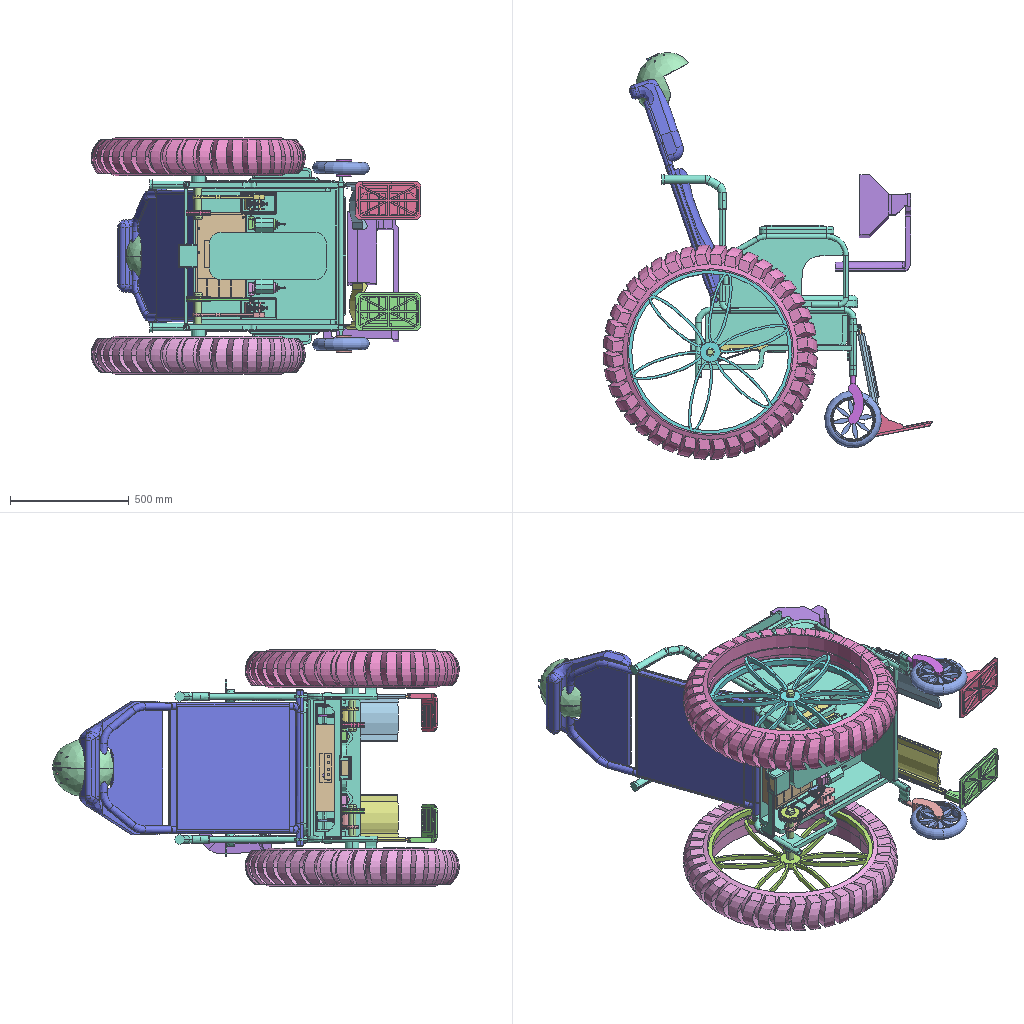Assembly | SolidWorks | 32 different items | 147 placed | box 1385 x 1709 x 995 mm
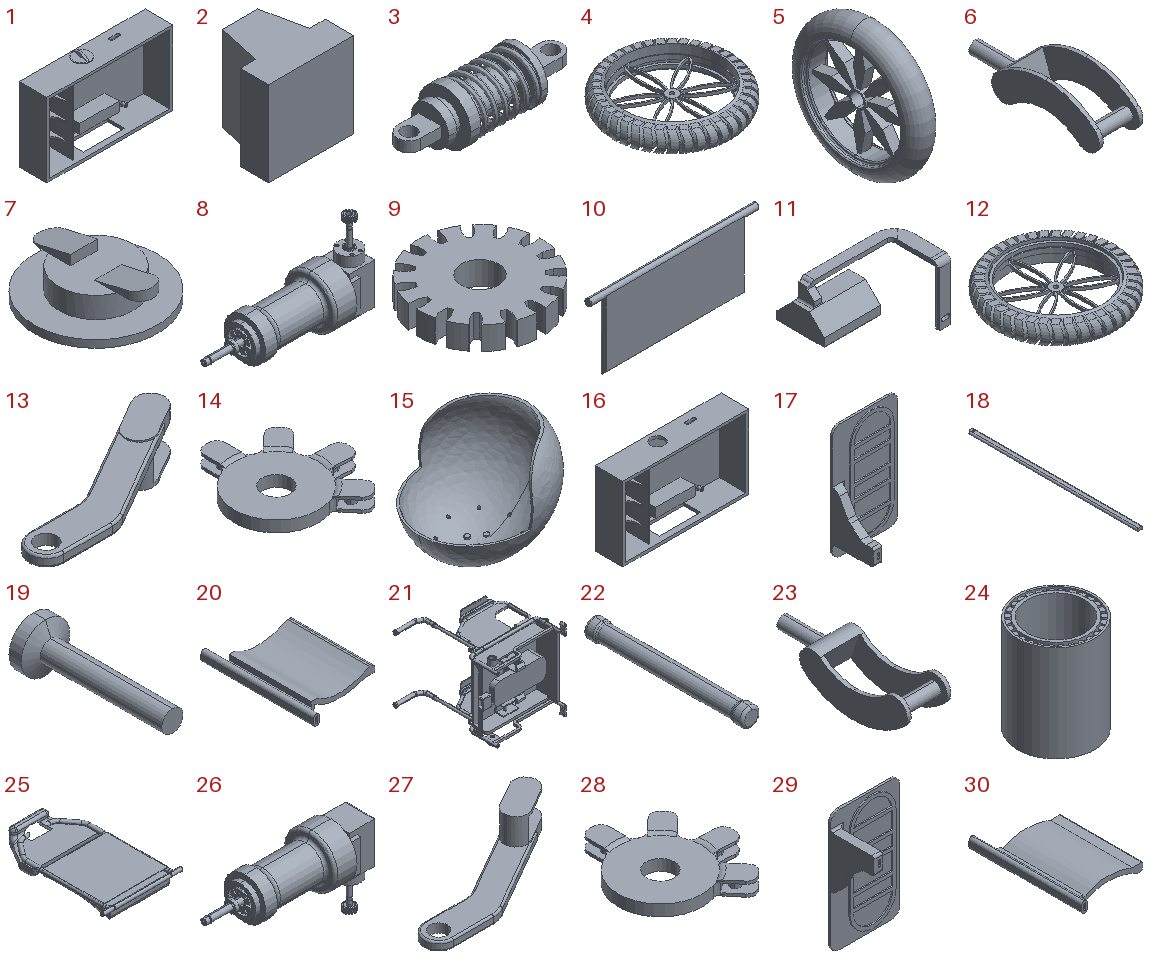Parts list (item | name | quantity | parent item | size | volume | features):
1 | (subassembly) | x1 | - | 366 x 80 x 226.454 mm | 995673 mm3 | features Fillet 2
2 | - | x109 | - | 6 x 5 x 6 mm | 128.419 mm3 | features Extrusion 1
3 | - | x2 | - | 79 x 25 x 25 mm | 12692 mm3 | features Extrusion 1, Helix 1, Revolution 1, Sweep 1
4 | - | x1 | - | 900 x 900 x 159.998 mm | 29745810 mm3 | features ICE 5, CirPattern 4, BossThin 1, ExtruThin 1, Fillet 1, RefAxis 1, RevCut 1, Revolution 1
5 | - | x2 | - | 50 x 239.862 x 239.862 mm | 1028496 mm3 | features ICE 3, CirPattern 1, Fillet 1, Revolution 1
6 | - | x1 | - | 69 x 230 x 64.48 mm | 170507 mm3 | features ICE 4, Extrusion 1
7 | - | x1 | in 1 | 50 x 50 x 22.954 mm | 14058 mm3 | features ICE 5, Extrusion 1
8 | - | x1 | - | 159.542 x 53.214 x 87.607 mm | 170177 mm3 | features ICE 20, Fillet 3, HoleWzd 2, CirPattern 1, Revolution 1
9 | - | x1 | - | 26.541 x 26.503 x 5 mm | 2075 mm3 | features ICE 4, CirPattern 1, Extrusion 1
10 | - | x1 | - | 79.5 x 3 x 34.5 mm | 6609 mm3 | features Fillet 2, Chamfer 1, Extrusion 1, ICE 1
11 | - | x1 | - | 546.764 x 377.712 x 317.016 mm | 9050376 mm3 | features ICE 10, Fillet 8, Chamfer 2, Sweep 2, Extrusion 1
12 | - | x1 | - | 900 x 900 x 159.998 mm | 29746479 mm3 | features MirrorStock 1
13 | - | x1 | - | 287.553 x 138.722 x 62 mm | 231304 mm3 | features ICE 4, Extrusion 1, Fillet 1, LPattern 1
14 | - | x1 | - | 80.013 x 90.67 x 10 mm | 26380 mm3 | features ICE 4, Fillet 2, CirPattern 1, Extrusion 1
15 | - | x1 | - | 256.913 x 240.018 x 217.091 mm | 479956 mm3 | features ICE 4, Bending 1, Fillet 1, Revolution 1, Shell 1
16 | - | x1 | in 1 | 366 x 80 x 216 mm | 981778 mm3 | features ICE 13, BossThin 1, Extrusion 1, LPattern 1
17 | - | x1 | - | 160 x 115 x 280 mm | 478660 mm3 | features Fillet 5, ICE 4, BossThin 2, Chamfer 1, Extrusion 1
18 | - | x2 | - | 14 x 400 x 6 mm | 30370 mm3 | features ICE 2, Extrusion 1
19 | - | x1 | - | 8 x 22.9 x 8 mm | 317.503 mm3 | features Revolution 1
20 | - | x1 | - | 194.613 x 302 x 37.008 mm | 615517 mm3 | features ExtruThin 1, ICE 1
21 | - | x1 | - | 838.639 x 850 x 766 mm | 46006837 mm3 | features ICE 30, Fillet 19, MirrorPattern 15, Cut 6, Sweep 4, BossThin 2, Chamfer 2, LPattern 2, MirrorSolid 1
22 | - | x2 | - | 35 x 300 x 35 mm | 221656 mm3 | features Fillet 3, Extrusion 1, ICE 1, MirrorPattern 1
23 | - | x1 | - | 69 x 230 x 64.48 mm | 170507 mm3 | features MirrorStock 1
24 | - | x2 | - | 40 x 40 x 50 mm | 21973 mm3 | features ICE 2, Extrusion 1
25 | - | x1 | - | 660 x 980.123 x 156.408 mm | 26120441 mm3 | features ICE 6, Fillet 4, Sweep 2, BossThin 1, Cut 1
26 | - | x1 | - | 159.542 x 53.214 x 87.607 mm | 170177 mm3 | features MirrorStock 1
27 | - | x1 | - | 287.553 x 138.722 x 62 mm | 231304 mm3 | features MirrorStock 1
28 | - | x1 | - | 80.013 x 90.67 x 10 mm | 26380 mm3 | features MirrorStock 1
29 | - | x1 | - | 160 x 115 x 280 mm | 478660 mm3 | features MirrorStock 1
30 | - | x1 | - | 194.613 x 302 x 37.008 mm | 615517 mm3 | features MirrorStock 1
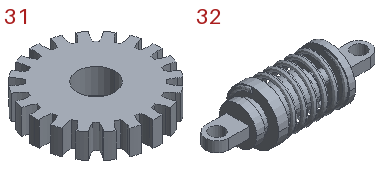31 | - | x2 | - | 99.281 x 99.281 x 20 mm | 114594 mm3 | features ICE 2, CirPattern 1, Cut 1, Extrusion 1
32 | - | x2 | - | 79 x 25 x 25 mm | 12692 mm3 | features MirrorStock 1
Mates (type | each side: item.copy, entity, surface, feature):
In the top assembly
Concentric | 6.1 face cylinder Boss-Extrude2 | 5.1 face cylinder Boss-Extrude2
Width | 6.1 face plane Boss-Extrude1 | 6.1 face plane Boss-Extrude1 | 5.1 face plane Boss-Extrude1 | 5.1 face plane Boss-Extrude1
Width | 21.1 face plane Boss-Extrude5 | 21.1 face plane Boss-Extrude5 | 18.1 face plane Boss-Extrude1 | 18.1 face plane Boss-Extrude1
Concentric | 21.1 face cylinder Cut-Extrude1 | 18.1 face cylinder Cut-Extrude2
DistanceDim | 6.1 face plane Boss-Extrude3 | 21.1 face plane Mirror3
Concentric | 18.1 face cylinder Cut-Extrude2 | 19.1 face cylinder Revolve1
DistanceDim | 19.1 face plane Revolve1 | 21.1 face plane Boss-Extrude5
Coincident | 17.1 face plane Cut-Extrude3 | 18.2 face plane Boss-Extrude1
Concentric | 17.1 face cylinder Cut-Extrude3 | 18.2 face cylinder Boss-Extrude1
DistanceDim | 17.1 face plane Cut-Extrude3 | 18.2 face plane Boss-Extrude1
Coincident | 18.1 face plane Boss-Extrude1 | 20.1 face plane Extrude-Thin1
Concentric | 18.1 face cylinder Boss-Extrude1 | 20.1 face cylinder Extrude-Thin1
DistanceDim | 29.1 face plane Footboard_Mirror | 20.1 face plane Extrude-Thin1
Concentric | 6.1 face cylinder Boss-Extrude3 | 21.1 face cylinder Mirror3
Concentric | 4.1 face cylinder Boss-Extrude1 | 21.1 face cylinder Mirror8
Concentric | 21.1 face cylinder Mirror8 | 24.1 face cylinder Boss-Extrude3
DistanceDim | 24.1 face plane Boss-Extrude1 | 21.1 face plane Boss-Extrude8
Concentric | 21.1 face cylinder Boss-Extrude15 | 25.1 face cylinder
Width | 25.1 face plane | 25.1 face plane | 21.1 face plane Mirror22 | 21.1 face plane Boss-Extrude15
DistanceDim | 4.1 face plane Boss-Extrude1 | 21.1 face plane Mirror7
Concentric | 4.1 face cylinder Boss-Extrude1 | 22.1 face cylinder Boss-Extrude1
Concentric | 21.1 face cylinder Cut-Extrude5 | 10.1 face cylinder Boss-Extrude2
Width | 21.1 face plane Boss-Extrude16 | 21.1 face plane Boss-Extrude16 | 10.1 face plane Boss-Extrude1 | 10.1 face plane Boss-Extrude1
Width | 11.1 face plane Cut-Extrude3 | 11.1 face plane Cut-Extrude3 | 21.1 face plane Sweep-Thin2 | 21.1 face plane Sweep-Thin2
DistanceDim | 4.1 face plane Boss-Extrude1 | 22.1 face plane Mirror1
Concentric | 22.1 face cylinder Boss-Extrude1 | 13.1 face cylinder Cut-Extrude1
DistanceDim | 21.1 face plane Boss-Extrude8 | 13.1 face plane Boss-Extrude1
Concentric | 3.1 face cylinder Boss-Extrude1 | 13.1 face cylinder Boss-Extrude3
Concentric | 13.1 face cylinder LPattern1 | 3.2 face cylinder Boss-Extrude1
Width | 13.1 face plane Cut-Extrude3 | 13.1 face plane Cut-Extrude3 | 3.2 face plane Boss-Extrude1 | 3.2 face plane Boss-Extrude1
Concentric | 22.1 face cylinder Boss-Extrude2 | 31.1 face cylinder Cut-Extrude1
Concentric | 3.1 face cylinder Boss-Extrude1 | 14.1 face cylinder CirPattern6
Concentric | 3.2 face cylinder Boss-Extrude1 | 14.1 face cylinder CirPattern6
Coincident | 21.1 face plane Cut-Extrude11 | 8.1 face plane Boss-Extrude3
Coincident | 21.1 face plane Boss-Extrude23 | 8.1 face plane Revolve1
Width | 14.1 face plane CirPattern6 | 14.1 face plane CirPattern6 | 3.2 face plane Boss-Extrude1 | 3.2 face plane Boss-Extrude1
Width | 13.1 face plane Cut-Extrude3 | 13.1 face plane Cut-Extrude3 | 3.1 face plane Boss-Extrude1 | 3.1 face plane Boss-Extrude1
Concentric | 21.1 face cylinder Mirror25 | 14.1 face cylinder Cut-Extrude1
DistanceDim | 13.1 face plane Boss-Extrude1 | 31.1 face plane Boss-Extrude1
DistanceDim | 16.1 face plane Boss-Extrude1 | 21.1 face plane Boss-Extrude18
Coincident | 21.1 face plane Boss-Extrude18 | 16.1 face plane Boss-Extrude1
Width | 16.1 face plane Boss-Extrude1 | 16.1 face plane Boss-Extrude1 | 21.1 face plane Boss-Extrude26 | 21.1 face plane Boss-Extrude26
Width | 31.1 face plane Boss-Extrude1 | 31.1 face plane Boss-Extrude1 | 9.1 face plane Boss-Extrude1 | 9.1 face plane Boss-Extrude1
Concentric | 9.1 face cylinder Cut-Extrude4 | assembly select_type:11
Concentric | 31.1 face cylinder Cut-Extrude1 | assembly select_type:11
BeltDim | 9.1 face cylinder Cut-Extrude3 | 31.1 face cylinder Cut-Extrude4
RackPinionDim | 2.1 edge | 9.1 face cylinder Cut-Extrude3
Coincident | 15.1 plane | assembly plane
Lock | 25.1 select_type:0 | 15.1 select_type:0
In subassembly 1
Coincident | 16.2 face plane Boss-Extrude1 | 7.1 face plane
Concentric | 16.2 face cylinder Cut-Extrude6 | 7.1 face cylinder